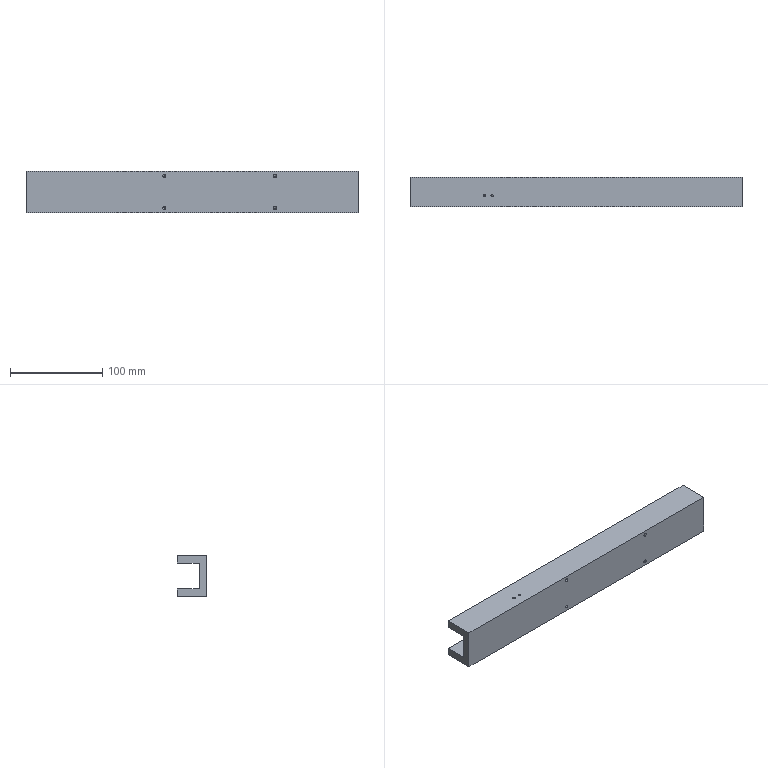Part | STEP file | PN_0028 | 1 solid | 74 faces | box 360 x 31.8 x 45 mm | volume 274443 mm3 | cylinder 32 | cone 32 | plane 10 | commonest cylinder face diameters 2.5 x24 3.3 x8